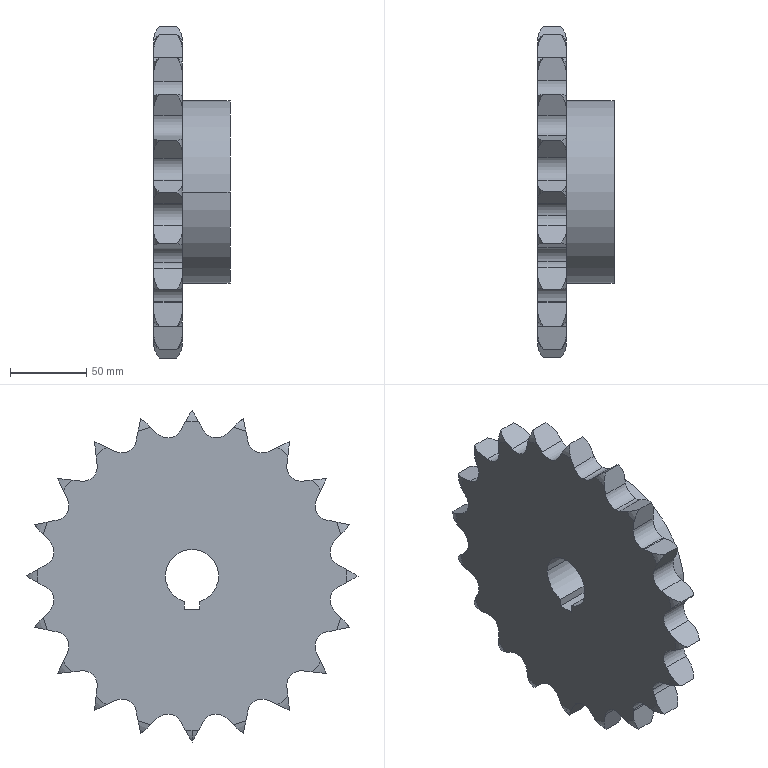Part | STEP file | IN-01-20-02 | 1 solid | 118 faces | box 50 x 218.1 x 218.1 mm | volume 860635 mm3 | plane 46 | spline 42 | cylinder 30 | commonest cylinder face diameters 19.05 x25 35 x3 120 x2